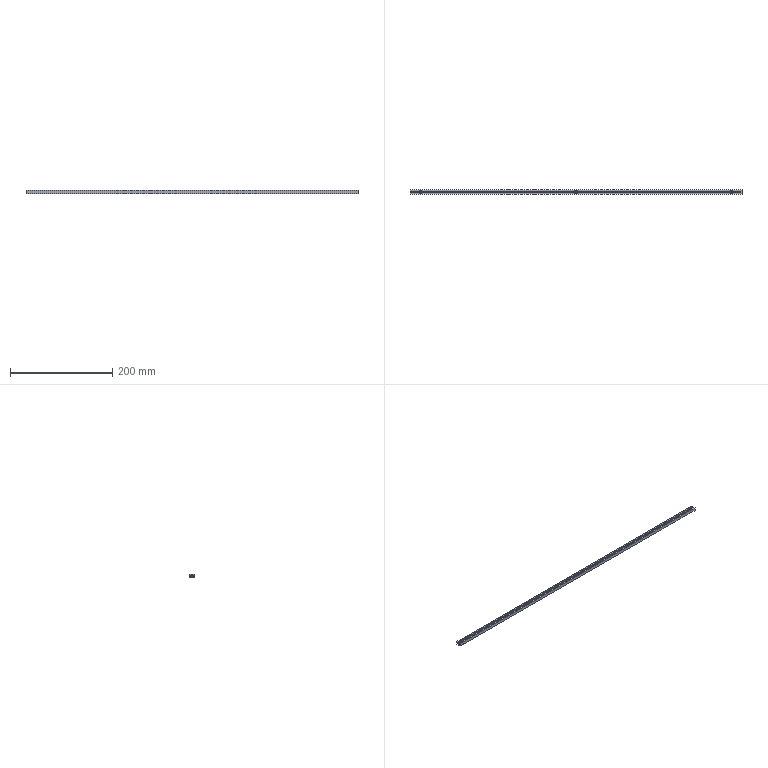Part | STEP file | 001-010-SENAM33H-650-V20-W325-X630 | 1 solid | 56 faces | box 650 x 9 x 6 mm | volume 20498 mm3 | plane 44 | cylinder 6 | cone 6 | commonest cylinder face diameters 6 x6